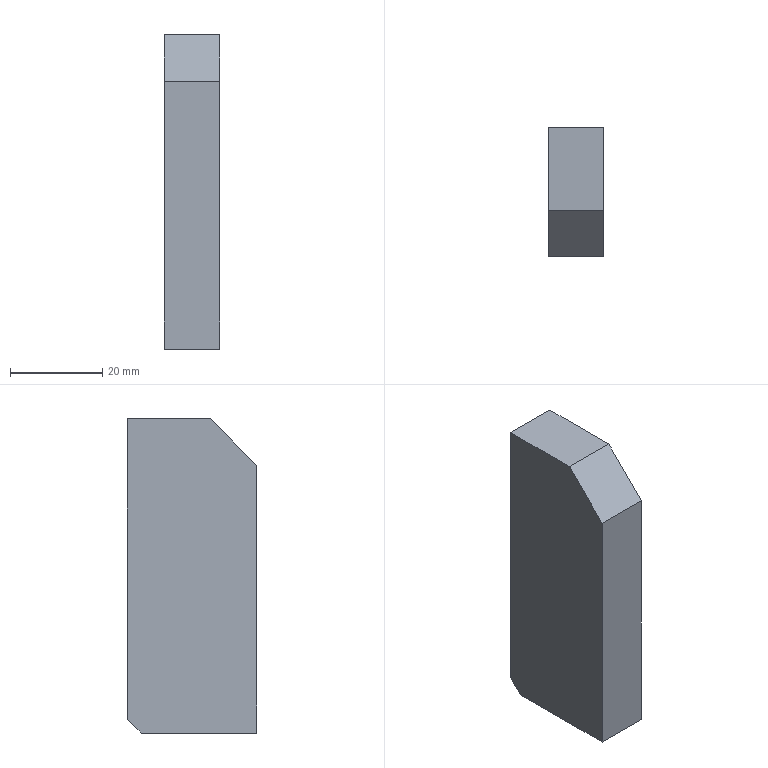Part | SolidWorks | features Chamfer 2, HoleWzd 2, Extrusion 1 | 1 solid | 24 faces | box 12 x 28 x 68 mm | volume 21134 mm3 | cylinder 8 | cone 8 | plane 8 | commonest cylinder face diameters 5 x8
STEP:
#1=CARTESIAN_POINT('',(-244.956,-13.,55.5));
#2=VERTEX_POINT('',#1);
#3=CARTESIAN_POINT('',(-244.956,-13.,60.5));
#4=VERTEX_POINT('',#3);
#5=CARTESIAN_POINT('',(-244.956,-13.,58.));
#6=DIRECTION('',(0.,1.,0.));
#7=DIRECTION('',(0.,0.,1.));
#8=AXIS2_PLACEMENT_3D('',#5,#6,#7);
#9=CIRCLE('',#8,2.5);
#10=EDGE_CURVE('',#2,#4,#9,.T.);
#11=ORIENTED_EDGE('',*,*,#10,.F.);
#12=CARTESIAN_POINT('',(-244.956,0.,55.5));
#13=VERTEX_POINT('',#12);
#14=CARTESIAN_POINT('',(-244.956,0.,55.5));
#15=DIRECTION('',(0.,1.,0.));
#16=VECTOR('',#15,1000.);
#17=LINE('',#14,#16);
#18=EDGE_CURVE('',#2,#13,#17,.T.);
#19=ORIENTED_EDGE('',*,*,#18,.T.);
#20=CARTESIAN_POINT('',(-244.956,0.,60.5));
#21=VERTEX_POINT('',#20);
#22=CARTESIAN_POINT('',(-244.956,0.,58.));
#23=DIRECTION('',(0.,1.,0.));
#24=DIRECTION('',(0.,0.,1.));
#25=AXIS2_PLACEMENT_3D('',#22,#23,#24);
#26=CIRCLE('',#25,2.5);
#27=EDGE_CURVE('',#13,#21,#26,.T.);
#28=ORIENTED_EDGE('',*,*,#27,.T.);
#29=CARTESIAN_POINT('',(-244.956,0.,60.5));
#30=DIRECTION('',(0.,1.,0.));
#31=VECTOR('',#30,1000.);
#32=LINE('',#29,#31);
#33=EDGE_CURVE('',#4,#21,#32,.T.);
#34=ORIENTED_EDGE('',*,*,#33,.F.);
#35=EDGE_LOOP('',(#11,#19,#28,#34));
#36=FACE_OUTER_BOUND('',#35,.T.);
#37=CARTESIAN_POINT('',(-244.956,0.,58.));
#38=DIRECTION('',(0.,1.,0.));
#39=DIRECTION('',(0.,0.,1.));
#40=AXIS2_PLACEMENT_3D('',#37,#38,#39);
#41=CYLINDRICAL_SURFACE('',#40,2.5);
#42=ADVANCED_FACE('',(#36),#41,.F.);
#43=CARTESIAN_POINT('',(-244.956,-14.502,58.));
#44=VERTEX_POINT('',#43);
#45=CARTESIAN_POINT('',(-244.956,-13.,60.5));
#46=DIRECTION('',(0.,0.515,0.8572));
#47=VECTOR('',#46,1000.);
#48=LINE('',#45,#47);
#49=EDGE_CURVE('',#44,#4,#48,.T.);
#50=ORIENTED_EDGE('',*,*,#49,.F.);
#51=CARTESIAN_POINT('',(-244.956,-13.,55.5));
#52=DIRECTION('',(0.,0.515,-0.8572));
#53=VECTOR('',#52,1000.);
#54=LINE('',#51,#53);
#55=EDGE_CURVE('',#44,#2,#54,.T.);
#56=ORIENTED_EDGE('',*,*,#55,.T.);
#57=ORIENTED_EDGE('',*,*,#10,.T.);
#58=EDGE_LOOP('',(#50,#56,#57));
#59=FACE_OUTER_BOUND('',#58,.T.);
#60=CARTESIAN_POINT('',(-244.956,-13.,58.));
#61=DIRECTION('',(0.,1.,0.));
#62=DIRECTION('',(0.,0.,1.));
#63=AXIS2_PLACEMENT_3D('',#60,#61,#62);
#64=CONICAL_SURFACE('',#63,2.5,1.03);
#65=ADVANCED_FACE('',(#59),#64,.F.);
#66=CARTESIAN_POINT('',(-244.956,-13.,17.5));
#67=VERTEX_POINT('',#66);
#68=CARTESIAN_POINT('',(-244.956,-13.,22.5));
#69=VERTEX_POINT('',#68);
#70=CARTESIAN_POINT('',(-244.956,-13.,20.));
#71=DIRECTION('',(0.,1.,0.));
#72=DIRECTION('',(0.,0.,1.));
#73=AXIS2_PLACEMENT_3D('',#70,#71,#72);
#74=CIRCLE('',#73,2.5);
#75=EDGE_CURVE('',#67,#69,#74,.T.);
#76=ORIENTED_EDGE('',*,*,#75,.F.);
#77=CARTESIAN_POINT('',(-244.956,0.,17.5));
#78=VERTEX_POINT('',#77);
#79=CARTESIAN_POINT('',(-244.956,0.,17.5));
#80=DIRECTION('',(0.,1.,0.));
#81=VECTOR('',#80,1000.);
#82=LINE('',#79,#81);
#83=EDGE_CURVE('',#67,#78,#82,.T.);
#84=ORIENTED_EDGE('',*,*,#83,.T.);
#85=CARTESIAN_POINT('',(-244.956,0.,22.5));
#86=VERTEX_POINT('',#85);
#87=CARTESIAN_POINT('',(-244.956,0.,20.));
#88=DIRECTION('',(0.,1.,0.));
#89=DIRECTION('',(0.,0.,1.));
#90=AXIS2_PLACEMENT_3D('',#87,#88,#89);
#91=CIRCLE('',#90,2.5);
#92=EDGE_CURVE('',#78,#86,#91,.T.);
#93=ORIENTED_EDGE('',*,*,#92,.T.);
#94=CARTESIAN_POINT('',(-244.956,0.,22.5));
#95=DIRECTION('',(0.,1.,0.));
#96=VECTOR('',#95,1000.);
#97=LINE('',#94,#96);
#98=EDGE_CURVE('',#69,#86,#97,.T.);
#99=ORIENTED_EDGE('',*,*,#98,.F.);
#100=EDGE_LOOP('',(#76,#84,#93,#99));
#101=FACE_OUTER_BOUND('',#100,.T.);
#102=CARTESIAN_POINT('',(-244.956,0.,20.));
#103=DIRECTION('',(0.,1.,0.));
#104=DIRECTION('',(0.,0.,1.));
#105=AXIS2_PLACEMENT_3D('',#102,#103,#104);
#106=CYLINDRICAL_SURFACE('',#105,2.5);
#107=ADVANCED_FACE('',(#101),#106,.F.);
#108=CARTESIAN_POINT('',(-244.956,-14.502,20.));
#109=VERTEX_POINT('',#108);
#110=CARTESIAN_POINT('',(-244.956,-13.,22.5));
#111=DIRECTION('',(0.,0.515,0.8572));
#112=VECTOR('',#111,1000.);
#113=LINE('',#110,#112);
#114=EDGE_CURVE('',#109,#69,#113,.T.);
#115=ORIENTED_EDGE('',*,*,#114,.F.);
#116=CARTESIAN_POINT('',(-244.956,-13.,17.5));
#117=DIRECTION('',(0.,0.515,-0.8572));
#118=VECTOR('',#117,1000.);
#119=LINE('',#116,#118);
#120=EDGE_CURVE('',#109,#67,#119,.T.);
#121=ORIENTED_EDGE('',*,*,#120,.T.);
#122=ORIENTED_EDGE('',*,*,#75,.T.);
#123=EDGE_LOOP('',(#115,#121,#122));
#124=FACE_OUTER_BOUND('',#123,.T.);
#125=CARTESIAN_POINT('',(-244.956,-13.,20.));
#126=DIRECTION('',(0.,1.,0.));
#127=DIRECTION('',(0.,0.,1.));
#128=AXIS2_PLACEMENT_3D('',#125,#126,#127);
#129=CONICAL_SURFACE('',#128,2.5,1.03);
#130=ADVANCED_FACE('',(#124),#129,.F.);
#131=CARTESIAN_POINT('',(-242.456,-9.,13.));
#132=VERTEX_POINT('',#131);
#133=CARTESIAN_POINT('',(-247.456,-9.,13.));
#134=VERTEX_POINT('',#133);
#135=CARTESIAN_POINT('',(-244.956,-9.,13.));
#136=DIRECTION('',(0.,0.,-1.));
#137=DIRECTION('',(-1.,0.,0.));
#138=AXIS2_PLACEMENT_3D('',#135,#136,#137);
#139=CIRCLE('',#138,2.5);
#140=EDGE_CURVE('',#132,#134,#139,.T.);
#141=ORIENTED_EDGE('',*,*,#140,.F.);
#142=CARTESIAN_POINT('',(-242.456,-9.,0.));
#143=VERTEX_POINT('',#142);
#144=CARTESIAN_POINT('',(-242.456,-9.,0.));
#145=DIRECTION('',(0.,0.,-1.));
#146=VECTOR('',#145,1000.);
#147=LINE('',#144,#146);
#148=EDGE_CURVE('',#132,#143,#147,.T.);
#149=ORIENTED_EDGE('',*,*,#148,.T.);
#150=CARTESIAN_POINT('',(-247.456,-9.,0.));
#151=VERTEX_POINT('',#150);
#152=CARTESIAN_POINT('',(-244.956,-9.,0.));
#153=DIRECTION('',(0.,0.,-1.));
#154=DIRECTION('',(-1.,0.,0.));
#155=AXIS2_PLACEMENT_3D('',#152,#153,#154);
#156=CIRCLE('',#155,2.5);
#157=EDGE_CURVE('',#143,#151,#156,.T.);
#158=ORIENTED_EDGE('',*,*,#157,.T.);
#159=CARTESIAN_POINT('',(-247.456,-9.,0.));
#160=DIRECTION('',(0.,0.,-1.));
#161=VECTOR('',#160,1000.);
#162=LINE('',#159,#161);
#163=EDGE_CURVE('',#134,#151,#162,.T.);
#164=ORIENTED_EDGE('',*,*,#163,.F.);
#165=EDGE_LOOP('',(#141,#149,#158,#164));
#166=FACE_OUTER_BOUND('',#165,.T.);
#167=CARTESIAN_POINT('',(-244.956,-9.,0.));
#168=DIRECTION('',(0.,0.,-1.));
#169=DIRECTION('',(-1.,0.,0.));
#170=AXIS2_PLACEMENT_3D('',#167,#168,#169);
#171=CYLINDRICAL_SURFACE('',#170,2.5);
#172=ADVANCED_FACE('',(#166),#171,.F.);
#173=CARTESIAN_POINT('',(-244.956,-9.,14.502));
#174=VERTEX_POINT('',#173);
#175=CARTESIAN_POINT('',(-247.456,-9.,13.));
#176=DIRECTION('',(-0.8572,0.,-0.515));
#177=VECTOR('',#176,1000.);
#178=LINE('',#175,#177);
#179=EDGE_CURVE('',#174,#134,#178,.T.);
#180=ORIENTED_EDGE('',*,*,#179,.F.);
#181=CARTESIAN_POINT('',(-242.456,-9.,13.));
#182=DIRECTION('',(0.8572,0.,-0.515));
#183=VECTOR('',#182,1000.);
#184=LINE('',#181,#183);
#185=EDGE_CURVE('',#174,#132,#184,.T.);
#186=ORIENTED_EDGE('',*,*,#185,.T.);
#187=ORIENTED_EDGE('',*,*,#140,.T.);
#188=EDGE_LOOP('',(#180,#186,#187));
#189=FACE_OUTER_BOUND('',#188,.T.);
#190=CARTESIAN_POINT('',(-244.956,-9.,13.));
#191=DIRECTION('',(0.,0.,-1.));
#192=DIRECTION('',(-1.,0.,0.));
#193=AXIS2_PLACEMENT_3D('',#190,#191,#192);
#194=CONICAL_SURFACE('',#193,2.5,1.03);
#195=ADVANCED_FACE('',(#189),#194,.F.);
#196=CARTESIAN_POINT('',(-242.456,-21.,13.));
#197=VERTEX_POINT('',#196);
#198=CARTESIAN_POINT('',(-247.456,-21.,13.));
#199=VERTEX_POINT('',#198);
#200=CARTESIAN_POINT('',(-244.956,-21.,13.));
#201=DIRECTION('',(0.,0.,-1.));
#202=DIRECTION('',(-1.,0.,0.));
#203=AXIS2_PLACEMENT_3D('',#200,#201,#202);
#204=CIRCLE('',#203,2.5);
#205=EDGE_CURVE('',#197,#199,#204,.T.);
#206=ORIENTED_EDGE('',*,*,#205,.F.);
#207=CARTESIAN_POINT('',(-242.456,-21.,0.));
#208=VERTEX_POINT('',#207);
#209=CARTESIAN_POINT('',(-242.456,-21.,0.));
#210=DIRECTION('',(0.,0.,-1.));
#211=VECTOR('',#210,1000.);
#212=LINE('',#209,#211);
#213=EDGE_CURVE('',#197,#208,#212,.T.);
#214=ORIENTED_EDGE('',*,*,#213,.T.);
#215=CARTESIAN_POINT('',(-247.456,-21.,0.));
#216=VERTEX_POINT('',#215);
#217=CARTESIAN_POINT('',(-244.956,-21.,0.));
#218=DIRECTION('',(0.,0.,-1.));
#219=DIRECTION('',(-1.,0.,0.));
#220=AXIS2_PLACEMENT_3D('',#217,#218,#219);
#221=CIRCLE('',#220,2.5);
#222=EDGE_CURVE('',#208,#216,#221,.T.);
#223=ORIENTED_EDGE('',*,*,#222,.T.);
#224=CARTESIAN_POINT('',(-247.456,-21.,0.));
#225=DIRECTION('',(0.,0.,-1.));
#226=VECTOR('',#225,1000.);
#227=LINE('',#224,#226);
#228=EDGE_CURVE('',#199,#216,#227,.T.);
#229=ORIENTED_EDGE('',*,*,#228,.F.);
#230=EDGE_LOOP('',(#206,#214,#223,#229));
#231=FACE_OUTER_BOUND('',#230,.T.);
#232=CARTESIAN_POINT('',(-244.956,-21.,0.));
#233=DIRECTION('',(0.,0.,-1.));
#234=DIRECTION('',(-1.,0.,0.));
#235=AXIS2_PLACEMENT_3D('',#232,#233,#234);
#236=CYLINDRICAL_SURFACE('',#235,2.5);
#237=ADVANCED_FACE('',(#231),#236,.F.);
#238=CARTESIAN_POINT('',(-244.956,-21.,14.502));
#239=VERTEX_POINT('',#238);
#240=CARTESIAN_POINT('',(-247.456,-21.,13.));
#241=DIRECTION('',(-0.8572,0.,-0.515));
#242=VECTOR('',#241,1000.);
#243=LINE('',#240,#242);
#244=EDGE_CURVE('',#239,#199,#243,.T.);
#245=ORIENTED_EDGE('',*,*,#244,.F.);
#246=CARTESIAN_POINT('',(-242.456,-21.,13.));
#247=DIRECTION('',(0.8572,0.,-0.515));
#248=VECTOR('',#247,1000.);
#249=LINE('',#246,#248);
#250=EDGE_CURVE('',#239,#197,#249,.T.);
#251=ORIENTED_EDGE('',*,*,#250,.T.);
#252=ORIENTED_EDGE('',*,*,#205,.T.);
#253=EDGE_LOOP('',(#245,#251,#252));
#254=FACE_OUTER_BOUND('',#253,.T.);
#255=CARTESIAN_POINT('',(-244.956,-21.,13.));
#256=DIRECTION('',(0.,0.,-1.));
#257=DIRECTION('',(-1.,0.,0.));
#258=AXIS2_PLACEMENT_3D('',#255,#256,#257);
#259=CONICAL_SURFACE('',#258,2.5,1.03);
#260=ADVANCED_FACE('',(#254),#259,.F.);
#261=CARTESIAN_POINT('',(-250.956,0.,68.));
#262=VERTEX_POINT('',#261);
#263=CARTESIAN_POINT('',(-250.956,0.,3.));
#264=VERTEX_POINT('',#263);
#265=CARTESIAN_POINT('',(-250.956,0.,68.));
#266=DIRECTION('',(0.,0.,-1.));
#267=VECTOR('',#266,1000.);
#268=LINE('',#265,#267);
#269=EDGE_CURVE('',#262,#264,#268,.T.);
#270=ORIENTED_EDGE('',*,*,#269,.T.);
#271=CARTESIAN_POINT('',(-250.956,-3.,0.));
#272=VERTEX_POINT('',#271);
#273=CARTESIAN_POINT('',(-250.956,0.,3.));
#274=DIRECTION('',(0.,-0.7071,-0.7071));
#275=VECTOR('',#274,1000.);
#276=LINE('',#273,#275);
#277=EDGE_CURVE('',#264,#272,#276,.T.);
#278=ORIENTED_EDGE('',*,*,#277,.T.);
#279=CARTESIAN_POINT('',(-250.956,-28.,0.));
#280=VERTEX_POINT('',#279);
#281=CARTESIAN_POINT('',(-250.956,0.,0.));
#282=DIRECTION('',(0.,-1.,0.));
#283=VECTOR('',#282,1000.);
#284=LINE('',#281,#283);
#285=EDGE_CURVE('',#272,#280,#284,.T.);
#286=ORIENTED_EDGE('',*,*,#285,.T.);
#287=CARTESIAN_POINT('',(-250.956,-28.,58.));
#288=VERTEX_POINT('',#287);
#289=CARTESIAN_POINT('',(-250.956,-28.,68.));
#290=DIRECTION('',(0.,0.,-1.));
#291=VECTOR('',#290,1000.);
#292=LINE('',#289,#291);
#293=EDGE_CURVE('',#288,#280,#292,.T.);
#294=ORIENTED_EDGE('',*,*,#293,.F.);
#295=CARTESIAN_POINT('',(-250.956,-18.,68.));
#296=VERTEX_POINT('',#295);
#297=CARTESIAN_POINT('',(-250.956,-18.,68.));
#298=DIRECTION('',(0.,0.7071,0.7071));
#299=VECTOR('',#298,1000.);
#300=LINE('',#297,#299);
#301=EDGE_CURVE('',#288,#296,#300,.T.);
#302=ORIENTED_EDGE('',*,*,#301,.T.);
#303=CARTESIAN_POINT('',(-250.956,0.,68.));
#304=DIRECTION('',(0.,-1.,0.));
#305=VECTOR('',#304,1000.);
#306=LINE('',#303,#305);
#307=EDGE_CURVE('',#262,#296,#306,.T.);
#308=ORIENTED_EDGE('',*,*,#307,.F.);
#309=EDGE_LOOP('',(#270,#278,#286,#294,#302,#308));
#310=FACE_OUTER_BOUND('',#309,.T.);
#311=CARTESIAN_POINT('',(-250.956,0.,68.));
#312=DIRECTION('',(1.,0.,0.));
#313=DIRECTION('',(0.,0.,-1.));
#314=AXIS2_PLACEMENT_3D('',#311,#312,#313);
#315=PLANE('',#314);
#316=ADVANCED_FACE('',(#310),#315,.F.);
#317=CARTESIAN_POINT('',(-238.956,-28.,58.));
#318=VERTEX_POINT('',#317);
#319=CARTESIAN_POINT('',(-238.956,-28.,0.));
#320=VERTEX_POINT('',#319);
#321=CARTESIAN_POINT('',(-238.956,-28.,68.));
#322=DIRECTION('',(0.,0.,-1.));
#323=VECTOR('',#322,1000.);
#324=LINE('',#321,#323);
#325=EDGE_CURVE('',#318,#320,#324,.T.);
#326=ORIENTED_EDGE('',*,*,#325,.F.);
#327=CARTESIAN_POINT('',(-250.956,-28.,58.));
#328=DIRECTION('',(-1.,0.,0.));
#329=VECTOR('',#328,1000.);
#330=LINE('',#327,#329);
#331=EDGE_CURVE('',#318,#288,#330,.T.);
#332=ORIENTED_EDGE('',*,*,#331,.T.);
#333=ORIENTED_EDGE('',*,*,#293,.T.);
#334=CARTESIAN_POINT('',(-250.956,-28.,0.));
#335=DIRECTION('',(1.,0.,0.));
#336=VECTOR('',#335,1000.);
#337=LINE('',#334,#336);
#338=EDGE_CURVE('',#280,#320,#337,.T.);
#339=ORIENTED_EDGE('',*,*,#338,.T.);
#340=EDGE_LOOP('',(#326,#332,#333,#339));
#341=FACE_OUTER_BOUND('',#340,.T.);
#342=CARTESIAN_POINT('',(-250.956,-28.,68.));
#343=DIRECTION('',(0.,1.,0.));
#344=DIRECTION('',(0.,0.,1.));
#345=AXIS2_PLACEMENT_3D('',#342,#343,#344);
#346=PLANE('',#345);
#347=ADVANCED_FACE('',(#341),#346,.F.);
#348=CARTESIAN_POINT('',(-238.956,-3.,0.));
#349=VERTEX_POINT('',#348);
#350=CARTESIAN_POINT('',(-238.956,0.,0.));
#351=DIRECTION('',(0.,1.,0.));
#352=VECTOR('',#351,1000.);
#353=LINE('',#350,#352);
#354=EDGE_CURVE('',#320,#349,#353,.T.);
#355=ORIENTED_EDGE('',*,*,#354,.T.);
#356=CARTESIAN_POINT('',(-238.956,0.,3.));
#357=VERTEX_POINT('',#356);
#358=CARTESIAN_POINT('',(-238.956,0.,3.));
#359=DIRECTION('',(0.,0.7071,0.7071));
#360=VECTOR('',#359,1000.);
#361=LINE('',#358,#360);
#362=EDGE_CURVE('',#349,#357,#361,.T.);
#363=ORIENTED_EDGE('',*,*,#362,.T.);
#364=CARTESIAN_POINT('',(-238.956,0.,68.));
#365=VERTEX_POINT('',#364);
#366=CARTESIAN_POINT('',(-238.956,0.,68.));
#367=DIRECTION('',(0.,0.,-1.));
#368=VECTOR('',#367,1000.);
#369=LINE('',#366,#368);
#370=EDGE_CURVE('',#365,#357,#369,.T.);
#371=ORIENTED_EDGE('',*,*,#370,.F.);
#372=CARTESIAN_POINT('',(-238.956,-18.,68.));
#373=VERTEX_POINT('',#372);
#374=CARTESIAN_POINT('',(-238.956,0.,68.));
#375=DIRECTION('',(0.,1.,0.));
#376=VECTOR('',#375,1000.);
#377=LINE('',#374,#376);
#378=EDGE_CURVE('',#373,#365,#377,.T.);
#379=ORIENTED_EDGE('',*,*,#378,.F.);
#380=CARTESIAN_POINT('',(-238.956,-18.,68.));
#381=DIRECTION('',(0.,-0.7071,-0.7071));
#382=VECTOR('',#381,1000.);
#383=LINE('',#380,#382);
#384=EDGE_CURVE('',#373,#318,#383,.T.);
#385=ORIENTED_EDGE('',*,*,#384,.T.);
#386=ORIENTED_EDGE('',*,*,#325,.T.);
#387=EDGE_LOOP('',(#355,#363,#371,#379,#385,#386));
#388=FACE_OUTER_BOUND('',#387,.T.);
#389=CARTESIAN_POINT('',(-238.956,0.,68.));
#390=DIRECTION('',(-1.,0.,0.));
#391=DIRECTION('',(0.,0.,1.));
#392=AXIS2_PLACEMENT_3D('',#389,#390,#391);
#393=PLANE('',#392);
#394=ADVANCED_FACE('',(#388),#393,.F.);
#395=CARTESIAN_POINT('',(-244.956,0.,58.));
#396=DIRECTION('',(0.,1.,0.));
#397=DIRECTION('',(0.,0.,1.));
#398=AXIS2_PLACEMENT_3D('',#395,#396,#397);
#399=CIRCLE('',#398,2.5);
#400=EDGE_CURVE('',#21,#13,#399,.T.);
#401=ORIENTED_EDGE('',*,*,#400,.F.);
#402=ORIENTED_EDGE('',*,*,#27,.F.);
#403=EDGE_LOOP('',(#401,#402));
#404=FACE_BOUND('',#403,.T.);
#405=CARTESIAN_POINT('',(-244.956,0.,20.));
#406=DIRECTION('',(0.,1.,0.));
#407=DIRECTION('',(0.,0.,1.));
#408=AXIS2_PLACEMENT_3D('',#405,#406,#407);
#409=CIRCLE('',#408,2.5);
#410=EDGE_CURVE('',#86,#78,#409,.T.);
#411=ORIENTED_EDGE('',*,*,#410,.F.);
#412=ORIENTED_EDGE('',*,*,#92,.F.);
#413=EDGE_LOOP('',(#411,#412));
#414=FACE_BOUND('',#413,.T.);
#415=ORIENTED_EDGE('',*,*,#370,.T.);
#416=CARTESIAN_POINT('',(-250.956,0.,3.));
#417=DIRECTION('',(-1.,0.,0.));
#418=VECTOR('',#417,1000.);
#419=LINE('',#416,#418);
#420=EDGE_CURVE('',#357,#264,#419,.T.);
#421=ORIENTED_EDGE('',*,*,#420,.T.);
#422=ORIENTED_EDGE('',*,*,#269,.F.);
#423=CARTESIAN_POINT('',(-250.956,0.,68.));
#424=DIRECTION('',(-1.,0.,0.));
#425=VECTOR('',#424,1000.);
#426=LINE('',#423,#425);
#427=EDGE_CURVE('',#365,#262,#426,.T.);
#428=ORIENTED_EDGE('',*,*,#427,.F.);
#429=EDGE_LOOP('',(#415,#421,#422,#428));
#430=FACE_OUTER_BOUND('',#429,.T.);
#431=CARTESIAN_POINT('',(-250.956,0.,68.));
#432=DIRECTION('',(0.,-1.,0.));
#433=DIRECTION('',(0.,0.,-1.));
#434=AXIS2_PLACEMENT_3D('',#431,#432,#433);
#435=PLANE('',#434);
#436=ADVANCED_FACE('',(#404,#414,#430),#435,.F.);
#437=ORIENTED_EDGE('',*,*,#307,.T.);
#438=CARTESIAN_POINT('',(-238.956,-18.,68.));
#439=DIRECTION('',(1.,0.,0.));
#440=VECTOR('',#439,1000.);
#441=LINE('',#438,#440);
#442=EDGE_CURVE('',#296,#373,#441,.T.);
#443=ORIENTED_EDGE('',*,*,#442,.T.);
#444=ORIENTED_EDGE('',*,*,#378,.T.);
#445=ORIENTED_EDGE('',*,*,#427,.T.);
#446=EDGE_LOOP('',(#437,#443,#444,#445));
#447=FACE_OUTER_BOUND('',#446,.T.);
#448=CARTESIAN_POINT('',(0.,0.,68.));
#449=DIRECTION('',(0.,0.,1.));
#450=DIRECTION('',(1.,0.,0.));
#451=AXIS2_PLACEMENT_3D('',#448,#449,#450);
#452=PLANE('',#451);
#453=ADVANCED_FACE('',(#447),#452,.T.);
#454=CARTESIAN_POINT('',(-244.956,-9.,0.));
#455=DIRECTION('',(0.,0.,-1.));
#456=DIRECTION('',(-1.,0.,0.));
#457=AXIS2_PLACEMENT_3D('',#454,#455,#456);
#458=CIRCLE('',#457,2.5);
#459=EDGE_CURVE('',#151,#143,#458,.T.);
#460=ORIENTED_EDGE('',*,*,#459,.F.);
#461=ORIENTED_EDGE('',*,*,#157,.F.);
#462=EDGE_LOOP('',(#460,#461));
#463=FACE_BOUND('',#462,.T.);
#464=CARTESIAN_POINT('',(-244.956,-21.,0.));
#465=DIRECTION('',(0.,0.,-1.));
#466=DIRECTION('',(-1.,0.,0.));
#467=AXIS2_PLACEMENT_3D('',#464,#465,#466);
#468=CIRCLE('',#467,2.5);
#469=EDGE_CURVE('',#216,#208,#468,.T.);
#470=ORIENTED_EDGE('',*,*,#469,.F.);
#471=ORIENTED_EDGE('',*,*,#222,.F.);
#472=EDGE_LOOP('',(#470,#471));
#473=FACE_BOUND('',#472,.T.);
#474=ORIENTED_EDGE('',*,*,#285,.F.);
#475=CARTESIAN_POINT('',(0.,-3.,0.));
#476=DIRECTION('',(1.,0.,0.));
#477=VECTOR('',#476,1000.);
#478=LINE('',#475,#477);
#479=EDGE_CURVE('',#272,#349,#478,.T.);
#480=ORIENTED_EDGE('',*,*,#479,.T.);
#481=ORIENTED_EDGE('',*,*,#354,.F.);
#482=ORIENTED_EDGE('',*,*,#338,.F.);
#483=EDGE_LOOP('',(#474,#480,#481,#482));
#484=FACE_OUTER_BOUND('',#483,.T.);
#485=CARTESIAN_POINT('',(0.,0.,0.));
#486=DIRECTION('',(0.,0.,1.));
#487=DIRECTION('',(1.,0.,0.));
#488=AXIS2_PLACEMENT_3D('',#485,#486,#487);
#489=PLANE('',#488);
#490=ADVANCED_FACE('',(#463,#473,#484),#489,.F.);
#491=ORIENTED_EDGE('',*,*,#301,.F.);
#492=ORIENTED_EDGE('',*,*,#331,.F.);
#493=ORIENTED_EDGE('',*,*,#384,.F.);
#494=ORIENTED_EDGE('',*,*,#442,.F.);
#495=EDGE_LOOP('',(#491,#492,#493,#494));
#496=FACE_OUTER_BOUND('',#495,.T.);
#497=CARTESIAN_POINT('',(0.,-18.,68.));
#498=DIRECTION('',(0.,-0.7071,0.7071));
#499=DIRECTION('',(-1.,0.,0.));
#500=AXIS2_PLACEMENT_3D('',#497,#498,#499);
#501=PLANE('',#500);
#502=ADVANCED_FACE('',(#496),#501,.T.);
#503=ORIENTED_EDGE('',*,*,#362,.F.);
#504=ORIENTED_EDGE('',*,*,#479,.F.);
#505=ORIENTED_EDGE('',*,*,#277,.F.);
#506=ORIENTED_EDGE('',*,*,#420,.F.);
#507=EDGE_LOOP('',(#503,#504,#505,#506));
#508=FACE_OUTER_BOUND('',#507,.T.);
#509=CARTESIAN_POINT('',(-250.956,0.,3.));
#510=DIRECTION('',(0.,-0.7071,0.7071));
#511=DIRECTION('',(-1.,0.,0.));
#512=AXIS2_PLACEMENT_3D('',#509,#510,#511);
#513=PLANE('',#512);
#514=ADVANCED_FACE('',(#508),#513,.F.);
#515=ORIENTED_EDGE('',*,*,#250,.F.);
#516=ORIENTED_EDGE('',*,*,#244,.T.);
#517=CARTESIAN_POINT('',(-244.956,-21.,13.));
#518=DIRECTION('',(0.,0.,-1.));
#519=DIRECTION('',(-1.,0.,0.));
#520=AXIS2_PLACEMENT_3D('',#517,#518,#519);
#521=CIRCLE('',#520,2.5);
#522=EDGE_CURVE('',#199,#197,#521,.T.);
#523=ORIENTED_EDGE('',*,*,#522,.T.);
#524=EDGE_LOOP('',(#515,#516,#523));
#525=FACE_OUTER_BOUND('',#524,.T.);
#526=CARTESIAN_POINT('',(-244.956,-21.,13.));
#527=DIRECTION('',(0.,0.,-1.));
#528=DIRECTION('',(-1.,0.,0.));
#529=AXIS2_PLACEMENT_3D('',#526,#527,#528);
#530=CONICAL_SURFACE('',#529,2.5,1.03);
#531=ADVANCED_FACE('',(#525),#530,.F.);
#532=ORIENTED_EDGE('',*,*,#213,.F.);
#533=ORIENTED_EDGE('',*,*,#522,.F.);
#534=ORIENTED_EDGE('',*,*,#228,.T.);
#535=ORIENTED_EDGE('',*,*,#469,.T.);
#536=EDGE_LOOP('',(#532,#533,#534,#535));
#537=FACE_OUTER_BOUND('',#536,.T.);
#538=CARTESIAN_POINT('',(-244.956,-21.,0.));
#539=DIRECTION('',(0.,0.,-1.));
#540=DIRECTION('',(-1.,0.,0.));
#541=AXIS2_PLACEMENT_3D('',#538,#539,#540);
#542=CYLINDRICAL_SURFACE('',#541,2.5);
#543=ADVANCED_FACE('',(#537),#542,.F.);
#544=ORIENTED_EDGE('',*,*,#185,.F.);
#545=ORIENTED_EDGE('',*,*,#179,.T.);
#546=CARTESIAN_POINT('',(-244.956,-9.,13.));
#547=DIRECTION('',(0.,0.,-1.));
#548=DIRECTION('',(-1.,0.,0.));
#549=AXIS2_PLACEMENT_3D('',#546,#547,#548);
#550=CIRCLE('',#549,2.5);
#551=EDGE_CURVE('',#134,#132,#550,.T.);
#552=ORIENTED_EDGE('',*,*,#551,.T.);
#553=EDGE_LOOP('',(#544,#545,#552));
#554=FACE_OUTER_BOUND('',#553,.T.);
#555=CARTESIAN_POINT('',(-244.956,-9.,13.));
#556=DIRECTION('',(0.,0.,-1.));
#557=DIRECTION('',(-1.,0.,0.));
#558=AXIS2_PLACEMENT_3D('',#555,#556,#557);
#559=CONICAL_SURFACE('',#558,2.5,1.03);
#560=ADVANCED_FACE('',(#554),#559,.F.);
#561=ORIENTED_EDGE('',*,*,#148,.F.);
#562=ORIENTED_EDGE('',*,*,#551,.F.);
#563=ORIENTED_EDGE('',*,*,#163,.T.);
#564=ORIENTED_EDGE('',*,*,#459,.T.);
#565=EDGE_LOOP('',(#561,#562,#563,#564));
#566=FACE_OUTER_BOUND('',#565,.T.);
#567=CARTESIAN_POINT('',(-244.956,-9.,0.));
#568=DIRECTION('',(0.,0.,-1.));
#569=DIRECTION('',(-1.,0.,0.));
#570=AXIS2_PLACEMENT_3D('',#567,#568,#569);
#571=CYLINDRICAL_SURFACE('',#570,2.5);
#572=ADVANCED_FACE('',(#566),#571,.F.);
#573=ORIENTED_EDGE('',*,*,#120,.F.);
#574=ORIENTED_EDGE('',*,*,#114,.T.);
#575=CARTESIAN_POINT('',(-244.956,-13.,20.));
#576=DIRECTION('',(0.,1.,0.));
#577=DIRECTION('',(0.,0.,1.));
#578=AXIS2_PLACEMENT_3D('',#575,#576,#577);
#579=CIRCLE('',#578,2.5);
#580=EDGE_CURVE('',#69,#67,#579,.T.);
#581=ORIENTED_EDGE('',*,*,#580,.T.);
#582=EDGE_LOOP('',(#573,#574,#581));
#583=FACE_OUTER_BOUND('',#582,.T.);
#584=CARTESIAN_POINT('',(-244.956,-13.,20.));
#585=DIRECTION('',(0.,1.,0.));
#586=DIRECTION('',(0.,0.,1.));
#587=AXIS2_PLACEMENT_3D('',#584,#585,#586);
#588=CONICAL_SURFACE('',#587,2.5,1.03);
#589=ADVANCED_FACE('',(#583),#588,.F.);
#590=ORIENTED_EDGE('',*,*,#83,.F.);
#591=ORIENTED_EDGE('',*,*,#580,.F.);
#592=ORIENTED_EDGE('',*,*,#98,.T.);
#593=ORIENTED_EDGE('',*,*,#410,.T.);
#594=EDGE_LOOP('',(#590,#591,#592,#593));
#595=FACE_OUTER_BOUND('',#594,.T.);
#596=CARTESIAN_POINT('',(-244.956,0.,20.));
#597=DIRECTION('',(0.,1.,0.));
#598=DIRECTION('',(0.,0.,1.));
#599=AXIS2_PLACEMENT_3D('',#596,#597,#598);
#600=CYLINDRICAL_SURFACE('',#599,2.5);
#601=ADVANCED_FACE('',(#595),#600,.F.);
#602=ORIENTED_EDGE('',*,*,#55,.F.);
#603=ORIENTED_EDGE('',*,*,#49,.T.);
#604=CARTESIAN_POINT('',(-244.956,-13.,58.));
#605=DIRECTION('',(0.,1.,0.));
#606=DIRECTION('',(0.,0.,1.));
#607=AXIS2_PLACEMENT_3D('',#604,#605,#606);
#608=CIRCLE('',#607,2.5);
#609=EDGE_CURVE('',#4,#2,#608,.T.);
#610=ORIENTED_EDGE('',*,*,#609,.T.);
#611=EDGE_LOOP('',(#602,#603,#610));
#612=FACE_OUTER_BOUND('',#611,.T.);
#613=CARTESIAN_POINT('',(-244.956,-13.,58.));
#614=DIRECTION('',(0.,1.,0.));
#615=DIRECTION('',(0.,0.,1.));
#616=AXIS2_PLACEMENT_3D('',#613,#614,#615);
#617=CONICAL_SURFACE('',#616,2.5,1.03);
#618=ADVANCED_FACE('',(#612),#617,.F.);
#619=ORIENTED_EDGE('',*,*,#18,.F.);
#620=ORIENTED_EDGE('',*,*,#609,.F.);
#621=ORIENTED_EDGE('',*,*,#33,.T.);
#622=ORIENTED_EDGE('',*,*,#400,.T.);
#623=EDGE_LOOP('',(#619,#620,#621,#622));
#624=FACE_OUTER_BOUND('',#623,.T.);
#625=CARTESIAN_POINT('',(-244.956,0.,58.));
#626=DIRECTION('',(0.,1.,0.));
#627=DIRECTION('',(0.,0.,1.));
#628=AXIS2_PLACEMENT_3D('',#625,#626,#627);
#629=CYLINDRICAL_SURFACE('',#628,2.5);
#630=ADVANCED_FACE('',(#624),#629,.F.);
#631=CLOSED_SHELL('',(#42,#65,#107,#130,#172,#195,#237,#260,#316,#347,#394,#436,#453,#490,#502,#514,#531,#543,#560,#572,#589,#601,#618,#630));
#632=MANIFOLD_SOLID_BREP('',#631);
#633=CARTESIAN_POINT('',(0.,0.,0.));
#634=DIRECTION('',(0.,0.,1.));
#635=DIRECTION('',(1.,0.,0.));
#636=AXIS2_PLACEMENT_3D('',#633,#634,#635);
#637=(LENGTH_UNIT()NAMED_UNIT(*)SI_UNIT(.MILLI.,.METRE.));
#638=UNCERTAINTY_MEASURE_WITH_UNIT(LENGTH_MEASURE(0.00001),#637,'','');
#639=(NAMED_UNIT(*)PLANE_ANGLE_UNIT()SI_UNIT($,.RADIAN.));
#640=(NAMED_UNIT(*)SI_UNIT($,.STERADIAN.)SOLID_ANGLE_UNIT());
#641=(GEOMETRIC_REPRESENTATION_CONTEXT(3)GLOBAL_UNCERTAINTY_ASSIGNED_CONTEXT((#638))GLOBAL_UNIT_ASSIGNED_CONTEXT((#637,#639,#640))REPRESENTATION_CONTEXT('',''));
#642=ADVANCED_BREP_SHAPE_REPRESENTATION('',(#632,#636),#641);